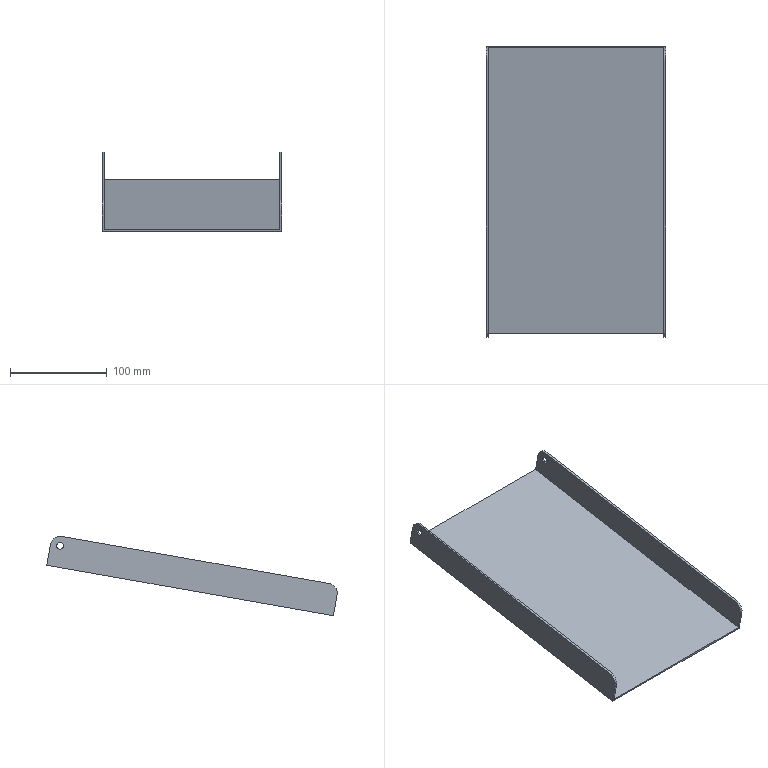Part | NX | features HB 2 | 1 solid | 16 faces | box 185 x 300.028 x 82.132 mm | volume 146980 mm3 | plane 10 | cylinder 6 | commonest cylinder face diameters 20 x4 7 x2
STEP:
#1=CARTESIAN_POINT('',(2913.,-963.709,-446.218));
#2=VERTEX_POINT('',#1);
#3=CARTESIAN_POINT('',(2913.,-687.349,-397.488));
#4=VERTEX_POINT('',#3);
#5=CARTESIAN_POINT('',(2913.,-562.892,-375.543));
#6=DIRECTION('',(0.,0.9848,0.1736));
#7=VECTOR('',#6,1000.);
#8=LINE('',#5,#7);
#9=EDGE_CURVE('',#2,#4,#8,.T.);
#10=ORIENTED_EDGE('',*,*,#9,.T.);
#11=CARTESIAN_POINT('',(2913.,-675.764,-405.6));
#12=VERTEX_POINT('',#11);
#13=CARTESIAN_POINT('',(2913.,-685.612,-407.336));
#14=DIRECTION('',(1.,0.,0.));
#15=DIRECTION('',(0.,-0.5736,0.8192));
#16=AXIS2_PLACEMENT_3D('',#13,#14,#15);
#17=CIRCLE('',#16,10.);
#18=EDGE_CURVE('',#12,#4,#17,.T.);
#19=ORIENTED_EDGE('',*,*,#18,.F.);
#20=CARTESIAN_POINT('',(2913.,-671.944,-427.266));
#21=VERTEX_POINT('',#20);
#22=CARTESIAN_POINT('',(2913.,-672.291,-425.296));
#23=DIRECTION('',(0.,-0.1736,0.9848));
#24=VECTOR('',#23,1000.);
#25=LINE('',#22,#24);
#26=EDGE_CURVE('',#21,#12,#25,.T.);
#27=ORIENTED_EDGE('',*,*,#26,.F.);
#28=CARTESIAN_POINT('',(2913.,-968.,-479.468));
#29=VERTEX_POINT('',#28);
#30=CARTESIAN_POINT('',(2913.,-557.335,-407.057));
#31=DIRECTION('',(0.,-0.9848,-0.1736));
#32=VECTOR('',#31,1000.);
#33=LINE('',#30,#32);
#34=EDGE_CURVE('',#21,#29,#33,.T.);
#35=ORIENTED_EDGE('',*,*,#34,.T.);
#36=CARTESIAN_POINT('',(2913.,-971.82,-457.803));
#37=VERTEX_POINT('',#36);
#38=CARTESIAN_POINT('',(2913.,-968.347,-477.499));
#39=DIRECTION('',(0.,-0.1736,0.9848));
#40=VECTOR('',#39,1000.);
#41=LINE('',#38,#40);
#42=EDGE_CURVE('',#29,#37,#41,.T.);
#43=ORIENTED_EDGE('',*,*,#42,.T.);
#44=CARTESIAN_POINT('',(2913.,-961.972,-456.066));
#45=DIRECTION('',(-1.,0.,0.));
#46=DIRECTION('',(0.,0.2588,0.9659));
#47=AXIS2_PLACEMENT_3D('',#44,#45,#46);
#48=CIRCLE('',#47,10.);
#49=EDGE_CURVE('',#37,#2,#48,.T.);
#50=ORIENTED_EDGE('',*,*,#49,.T.);
#51=EDGE_LOOP('',(#10,#19,#27,#35,#43,#50));
#52=FACE_BOUND('',#51,.T.);
#53=CARTESIAN_POINT('',(2913.,-684.707,-403.956));
#54=VERTEX_POINT('',#53);
#55=CARTESIAN_POINT('',(2913.,-685.612,-407.336));
#56=DIRECTION('',(1.,0.,0.));
#57=DIRECTION('',(0.,0.2588,0.9659));
#58=AXIS2_PLACEMENT_3D('',#55,#56,#57);
#59=CIRCLE('',#58,3.5);
#60=EDGE_CURVE('',#54,#54,#59,.T.);
#61=ORIENTED_EDGE('',*,*,#60,.T.);
#62=EDGE_LOOP('',(#61));
#63=FACE_BOUND('',#62,.T.);
#64=CARTESIAN_POINT('',(2913.,-557.683,-405.087));
#65=DIRECTION('',(1.,0.,0.));
#66=DIRECTION('',(0.,-0.2588,-0.9659));
#67=AXIS2_PLACEMENT_3D('',#64,#65,#66);
#68=PLANE('',#67);
#69=ADVANCED_FACE('',(#52,#63),#68,.F.);
#70=CARTESIAN_POINT('',(2915.,-963.709,-446.218));
#71=VERTEX_POINT('',#70);
#72=CARTESIAN_POINT('',(2915.,-971.82,-457.803));
#73=VERTEX_POINT('',#72);
#74=CARTESIAN_POINT('',(2915.,-961.972,-456.066));
#75=DIRECTION('',(1.,0.,0.));
#76=DIRECTION('',(0.,0.2588,0.9659));
#77=AXIS2_PLACEMENT_3D('',#74,#75,#76);
#78=CIRCLE('',#77,10.);
#79=EDGE_CURVE('',#71,#73,#78,.T.);
#80=ORIENTED_EDGE('',*,*,#79,.T.);
#81=CARTESIAN_POINT('',(2915.,-968.347,-477.499));
#82=VERTEX_POINT('',#81);
#83=CARTESIAN_POINT('',(2915.,-968.347,-477.499));
#84=DIRECTION('',(0.,-0.1736,0.9848));
#85=VECTOR('',#84,1000.);
#86=LINE('',#83,#85);
#87=EDGE_CURVE('',#82,#73,#86,.T.);
#88=ORIENTED_EDGE('',*,*,#87,.F.);
#89=CARTESIAN_POINT('',(2915.,-672.291,-425.296));
#90=VERTEX_POINT('',#89);
#91=CARTESIAN_POINT('',(2915.,-557.683,-405.087));
#92=DIRECTION('',(0.,0.9848,0.1736));
#93=VECTOR('',#92,1000.);
#94=LINE('',#91,#93);
#95=EDGE_CURVE('',#82,#90,#94,.T.);
#96=ORIENTED_EDGE('',*,*,#95,.T.);
#97=CARTESIAN_POINT('',(2915.,-675.764,-405.6));
#98=VERTEX_POINT('',#97);
#99=CARTESIAN_POINT('',(2915.,-672.291,-425.296));
#100=DIRECTION('',(0.,-0.1736,0.9848));
#101=VECTOR('',#100,1000.);
#102=LINE('',#99,#101);
#103=EDGE_CURVE('',#90,#98,#102,.T.);
#104=ORIENTED_EDGE('',*,*,#103,.T.);
#105=CARTESIAN_POINT('',(2915.,-687.349,-397.488));
#106=VERTEX_POINT('',#105);
#107=CARTESIAN_POINT('',(2915.,-685.612,-407.336));
#108=DIRECTION('',(-1.,0.,0.));
#109=DIRECTION('',(0.,-0.5736,0.8192));
#110=AXIS2_PLACEMENT_3D('',#107,#108,#109);
#111=CIRCLE('',#110,10.);
#112=EDGE_CURVE('',#106,#98,#111,.T.);
#113=ORIENTED_EDGE('',*,*,#112,.F.);
#114=CARTESIAN_POINT('',(2915.,-562.892,-375.543));
#115=DIRECTION('',(0.,0.9848,0.1736));
#116=VECTOR('',#115,1000.);
#117=LINE('',#114,#116);
#118=EDGE_CURVE('',#71,#106,#117,.T.);
#119=ORIENTED_EDGE('',*,*,#118,.F.);
#120=EDGE_LOOP('',(#80,#88,#96,#104,#113,#119));
#121=FACE_BOUND('',#120,.T.);
#122=CARTESIAN_POINT('',(2915.,-684.707,-403.956));
#123=VERTEX_POINT('',#122);
#124=CARTESIAN_POINT('',(2915.,-685.612,-407.336));
#125=DIRECTION('',(-1.,0.,0.));
#126=DIRECTION('',(0.,0.2588,0.9659));
#127=AXIS2_PLACEMENT_3D('',#124,#125,#126);
#128=CIRCLE('',#127,3.5);
#129=EDGE_CURVE('',#123,#123,#128,.T.);
#130=ORIENTED_EDGE('',*,*,#129,.T.);
#131=EDGE_LOOP('',(#130));
#132=FACE_BOUND('',#131,.T.);
#133=CARTESIAN_POINT('',(2915.,-557.683,-405.087));
#134=DIRECTION('',(1.,0.,0.));
#135=DIRECTION('',(0.,0.2588,0.9659));
#136=AXIS2_PLACEMENT_3D('',#133,#134,#135);
#137=PLANE('',#136);
#138=ADVANCED_FACE('',(#121,#132),#137,.T.);
#139=CARTESIAN_POINT('',(3098.,-686.518,-410.717));
#140=VERTEX_POINT('',#139);
#141=CARTESIAN_POINT('',(3098.,-685.612,-407.336));
#142=DIRECTION('',(-1.,0.,0.));
#143=DIRECTION('',(0.,-0.2588,-0.9659));
#144=AXIS2_PLACEMENT_3D('',#141,#142,#143);
#145=CIRCLE('',#144,3.5);
#146=EDGE_CURVE('',#140,#140,#145,.T.);
#147=ORIENTED_EDGE('',*,*,#146,.T.);
#148=EDGE_LOOP('',(#147));
#149=FACE_BOUND('',#148,.T.);
#150=CARTESIAN_POINT('',(3098.,-968.,-479.468));
#151=VERTEX_POINT('',#150);
#152=CARTESIAN_POINT('',(3098.,-671.944,-427.266));
#153=VERTEX_POINT('',#152);
#154=CARTESIAN_POINT('',(3098.,-557.335,-407.057));
#155=DIRECTION('',(0.,0.9848,0.1736));
#156=VECTOR('',#155,1000.);
#157=LINE('',#154,#156);
#158=EDGE_CURVE('',#151,#153,#157,.T.);
#159=ORIENTED_EDGE('',*,*,#158,.T.);
#160=CARTESIAN_POINT('',(3098.,-675.764,-405.6));
#161=VERTEX_POINT('',#160);
#162=CARTESIAN_POINT('',(3098.,-672.291,-425.296));
#163=DIRECTION('',(0.,-0.1736,0.9848));
#164=VECTOR('',#163,1000.);
#165=LINE('',#162,#164);
#166=EDGE_CURVE('',#153,#161,#165,.T.);
#167=ORIENTED_EDGE('',*,*,#166,.T.);
#168=CARTESIAN_POINT('',(3098.,-687.349,-397.488));
#169=VERTEX_POINT('',#168);
#170=CARTESIAN_POINT('',(3098.,-685.612,-407.336));
#171=DIRECTION('',(-1.,0.,0.));
#172=DIRECTION('',(0.,0.5736,-0.8192));
#173=AXIS2_PLACEMENT_3D('',#170,#171,#172);
#174=CIRCLE('',#173,10.);
#175=EDGE_CURVE('',#169,#161,#174,.T.);
#176=ORIENTED_EDGE('',*,*,#175,.F.);
#177=CARTESIAN_POINT('',(3098.,-963.709,-446.218));
#178=VERTEX_POINT('',#177);
#179=CARTESIAN_POINT('',(3098.,-562.892,-375.543));
#180=DIRECTION('',(0.,0.9848,0.1736));
#181=VECTOR('',#180,1000.);
#182=LINE('',#179,#181);
#183=EDGE_CURVE('',#178,#169,#182,.T.);
#184=ORIENTED_EDGE('',*,*,#183,.F.);
#185=CARTESIAN_POINT('',(3098.,-971.82,-457.803));
#186=VERTEX_POINT('',#185);
#187=CARTESIAN_POINT('',(3098.,-961.972,-456.066));
#188=DIRECTION('',(1.,0.,0.));
#189=DIRECTION('',(0.,-0.2588,-0.9659));
#190=AXIS2_PLACEMENT_3D('',#187,#188,#189);
#191=CIRCLE('',#190,10.);
#192=EDGE_CURVE('',#178,#186,#191,.T.);
#193=ORIENTED_EDGE('',*,*,#192,.T.);
#194=CARTESIAN_POINT('',(3098.,-968.347,-477.499));
#195=DIRECTION('',(0.,-0.1736,0.9848));
#196=VECTOR('',#195,1000.);
#197=LINE('',#194,#196);
#198=EDGE_CURVE('',#151,#186,#197,.T.);
#199=ORIENTED_EDGE('',*,*,#198,.F.);
#200=EDGE_LOOP('',(#159,#167,#176,#184,#193,#199));
#201=FACE_BOUND('',#200,.T.);
#202=CARTESIAN_POINT('',(3098.,-557.683,-405.087));
#203=DIRECTION('',(-1.,0.,0.));
#204=DIRECTION('',(0.,0.2588,0.9659));
#205=AXIS2_PLACEMENT_3D('',#202,#203,#204);
#206=PLANE('',#205);
#207=ADVANCED_FACE('',(#149,#201),#206,.F.);
#208=CARTESIAN_POINT('',(3096.,-968.347,-477.499));
#209=VERTEX_POINT('',#208);
#210=CARTESIAN_POINT('',(2994.,-968.347,-477.499));
#211=DIRECTION('',(1.,0.,0.));
#212=VECTOR('',#211,1000.);
#213=LINE('',#210,#212);
#214=EDGE_CURVE('',#82,#209,#213,.T.);
#215=ORIENTED_EDGE('',*,*,#214,.T.);
#216=CARTESIAN_POINT('',(3096.,-672.291,-425.296));
#217=VERTEX_POINT('',#216);
#218=CARTESIAN_POINT('',(3096.,-557.683,-405.087));
#219=DIRECTION('',(0.,-0.9848,-0.1736));
#220=VECTOR('',#219,1000.);
#221=LINE('',#218,#220);
#222=EDGE_CURVE('',#217,#209,#221,.T.);
#223=ORIENTED_EDGE('',*,*,#222,.F.);
#224=CARTESIAN_POINT('',(2994.,-672.291,-425.296));
#225=DIRECTION('',(1.,0.,0.));
#226=VECTOR('',#225,1000.);
#227=LINE('',#224,#226);
#228=EDGE_CURVE('',#90,#217,#227,.T.);
#229=ORIENTED_EDGE('',*,*,#228,.F.);
#230=ORIENTED_EDGE('',*,*,#95,.F.);
#231=EDGE_LOOP('',(#215,#223,#229,#230));
#232=FACE_BOUND('',#231,.T.);
#233=CARTESIAN_POINT('',(2994.,-557.683,-405.087));
#234=DIRECTION('',(0.,-0.1736,0.9848));
#235=DIRECTION('',(1.,0.,0.));
#236=AXIS2_PLACEMENT_3D('',#233,#234,#235);
#237=PLANE('',#236);
#238=ADVANCED_FACE('',(#232),#237,.T.);
#239=CARTESIAN_POINT('',(2994.,-671.944,-427.266));
#240=DIRECTION('',(1.,0.,0.));
#241=VECTOR('',#240,1000.);
#242=LINE('',#239,#241);
#243=EDGE_CURVE('',#21,#153,#242,.T.);
#244=ORIENTED_EDGE('',*,*,#243,.T.);
#245=ORIENTED_EDGE('',*,*,#158,.F.);
#246=CARTESIAN_POINT('',(2994.,-968.,-479.468));
#247=DIRECTION('',(1.,0.,0.));
#248=VECTOR('',#247,1000.);
#249=LINE('',#246,#248);
#250=EDGE_CURVE('',#29,#151,#249,.T.);
#251=ORIENTED_EDGE('',*,*,#250,.F.);
#252=ORIENTED_EDGE('',*,*,#34,.F.);
#253=EDGE_LOOP('',(#244,#245,#251,#252));
#254=FACE_BOUND('',#253,.T.);
#255=CARTESIAN_POINT('',(2994.,-557.335,-407.057));
#256=DIRECTION('',(0.,-0.1736,0.9848));
#257=DIRECTION('',(1.,0.,0.));
#258=AXIS2_PLACEMENT_3D('',#255,#256,#257);
#259=PLANE('',#258);
#260=ADVANCED_FACE('',(#254),#259,.F.);
#261=ORIENTED_EDGE('',*,*,#183,.T.);
#262=CARTESIAN_POINT('',(3096.,-687.349,-397.488));
#263=VERTEX_POINT('',#262);
#264=CARTESIAN_POINT('',(3226.,-687.349,-397.488));
#265=DIRECTION('',(1.,0.,0.));
#266=VECTOR('',#265,1000.);
#267=LINE('',#264,#266);
#268=EDGE_CURVE('',#263,#169,#267,.T.);
#269=ORIENTED_EDGE('',*,*,#268,.F.);
#270=CARTESIAN_POINT('',(3096.,-963.709,-446.218));
#271=VERTEX_POINT('',#270);
#272=CARTESIAN_POINT('',(3096.,-562.892,-375.543));
#273=DIRECTION('',(0.,0.9848,0.1736));
#274=VECTOR('',#273,1000.);
#275=LINE('',#272,#274);
#276=EDGE_CURVE('',#271,#263,#275,.T.);
#277=ORIENTED_EDGE('',*,*,#276,.F.);
#278=CARTESIAN_POINT('',(3226.,-963.709,-446.218));
#279=DIRECTION('',(1.,0.,0.));
#280=VECTOR('',#279,1000.);
#281=LINE('',#278,#280);
#282=EDGE_CURVE('',#271,#178,#281,.T.);
#283=ORIENTED_EDGE('',*,*,#282,.T.);
#284=EDGE_LOOP('',(#261,#269,#277,#283));
#285=FACE_BOUND('',#284,.T.);
#286=CARTESIAN_POINT('',(3226.,-562.892,-375.543));
#287=DIRECTION('',(0.,0.1736,-0.9848));
#288=DIRECTION('',(0.,-0.9848,-0.1736));
#289=AXIS2_PLACEMENT_3D('',#286,#287,#288);
#290=PLANE('',#289);
#291=ADVANCED_FACE('',(#285),#290,.F.);
#292=CARTESIAN_POINT('',(3096.,-686.518,-410.717));
#293=VERTEX_POINT('',#292);
#294=CARTESIAN_POINT('',(3096.,-685.612,-407.336));
#295=DIRECTION('',(-1.,0.,0.));
#296=DIRECTION('',(0.,-0.2588,-0.9659));
#297=AXIS2_PLACEMENT_3D('',#294,#295,#296);
#298=CIRCLE('',#297,3.5);
#299=EDGE_CURVE('',#293,#293,#298,.T.);
#300=ORIENTED_EDGE('',*,*,#299,.F.);
#301=EDGE_LOOP('',(#300));
#302=FACE_BOUND('',#301,.T.);
#303=ORIENTED_EDGE('',*,*,#222,.T.);
#304=CARTESIAN_POINT('',(3096.,-971.82,-457.803));
#305=VERTEX_POINT('',#304);
#306=CARTESIAN_POINT('',(3096.,-968.347,-477.499));
#307=DIRECTION('',(0.,-0.1736,0.9848));
#308=VECTOR('',#307,1000.);
#309=LINE('',#306,#308);
#310=EDGE_CURVE('',#209,#305,#309,.T.);
#311=ORIENTED_EDGE('',*,*,#310,.T.);
#312=CARTESIAN_POINT('',(3096.,-961.972,-456.066));
#313=DIRECTION('',(-1.,0.,0.));
#314=DIRECTION('',(0.,-0.2588,-0.9659));
#315=AXIS2_PLACEMENT_3D('',#312,#313,#314);
#316=CIRCLE('',#315,10.);
#317=EDGE_CURVE('',#305,#271,#316,.T.);
#318=ORIENTED_EDGE('',*,*,#317,.T.);
#319=ORIENTED_EDGE('',*,*,#276,.T.);
#320=CARTESIAN_POINT('',(3096.,-675.764,-405.6));
#321=VERTEX_POINT('',#320);
#322=CARTESIAN_POINT('',(3096.,-685.612,-407.336));
#323=DIRECTION('',(1.,0.,0.));
#324=DIRECTION('',(0.,0.5736,-0.8192));
#325=AXIS2_PLACEMENT_3D('',#322,#323,#324);
#326=CIRCLE('',#325,10.);
#327=EDGE_CURVE('',#321,#263,#326,.T.);
#328=ORIENTED_EDGE('',*,*,#327,.F.);
#329=CARTESIAN_POINT('',(3096.,-672.291,-425.296));
#330=DIRECTION('',(0.,-0.1736,0.9848));
#331=VECTOR('',#330,1000.);
#332=LINE('',#329,#331);
#333=EDGE_CURVE('',#217,#321,#332,.T.);
#334=ORIENTED_EDGE('',*,*,#333,.F.);
#335=EDGE_LOOP('',(#303,#311,#318,#319,#328,#334));
#336=FACE_BOUND('',#335,.T.);
#337=CARTESIAN_POINT('',(3096.,-557.683,-405.087));
#338=DIRECTION('',(-1.,0.,0.));
#339=DIRECTION('',(0.,0.2588,0.9659));
#340=AXIS2_PLACEMENT_3D('',#337,#338,#339);
#341=PLANE('',#340);
#342=ADVANCED_FACE('',(#302,#336),#341,.T.);
#343=ORIENTED_EDGE('',*,*,#118,.T.);
#344=CARTESIAN_POINT('',(2929.,-687.349,-397.488));
#345=DIRECTION('',(1.,0.,0.));
#346=VECTOR('',#345,1000.);
#347=LINE('',#344,#346);
#348=EDGE_CURVE('',#4,#106,#347,.T.);
#349=ORIENTED_EDGE('',*,*,#348,.F.);
#350=ORIENTED_EDGE('',*,*,#9,.F.);
#351=CARTESIAN_POINT('',(2929.,-963.709,-446.218));
#352=DIRECTION('',(1.,0.,0.));
#353=VECTOR('',#352,1000.);
#354=LINE('',#351,#353);
#355=EDGE_CURVE('',#2,#71,#354,.T.);
#356=ORIENTED_EDGE('',*,*,#355,.T.);
#357=EDGE_LOOP('',(#343,#349,#350,#356));
#358=FACE_BOUND('',#357,.T.);
#359=CARTESIAN_POINT('',(2929.,-562.892,-375.543));
#360=DIRECTION('',(0.,0.1736,-0.9848));
#361=DIRECTION('',(0.,-0.9848,-0.1736));
#362=AXIS2_PLACEMENT_3D('',#359,#360,#361);
#363=PLANE('',#362);
#364=ADVANCED_FACE('',(#358),#363,.F.);
#365=ORIENTED_EDGE('',*,*,#42,.F.);
#366=ORIENTED_EDGE('',*,*,#250,.T.);
#367=ORIENTED_EDGE('',*,*,#198,.T.);
#368=CARTESIAN_POINT('',(2994.,-971.82,-457.803));
#369=DIRECTION('',(-1.,0.,0.));
#370=VECTOR('',#369,1000.);
#371=LINE('',#368,#370);
#372=EDGE_CURVE('',#186,#305,#371,.T.);
#373=ORIENTED_EDGE('',*,*,#372,.T.);
#374=ORIENTED_EDGE('',*,*,#310,.F.);
#375=ORIENTED_EDGE('',*,*,#214,.F.);
#376=ORIENTED_EDGE('',*,*,#87,.T.);
#377=CARTESIAN_POINT('',(2994.,-971.82,-457.803));
#378=DIRECTION('',(-1.,0.,0.));
#379=VECTOR('',#378,1000.);
#380=LINE('',#377,#379);
#381=EDGE_CURVE('',#73,#37,#380,.T.);
#382=ORIENTED_EDGE('',*,*,#381,.T.);
#383=EDGE_LOOP('',(#365,#366,#367,#373,#374,#375,#376,#382));
#384=FACE_BOUND('',#383,.T.);
#385=CARTESIAN_POINT('',(2994.,-968.347,-477.499));
#386=DIRECTION('',(0.,0.9848,0.1736));
#387=DIRECTION('',(0.,0.1736,-0.9848));
#388=AXIS2_PLACEMENT_3D('',#385,#386,#387);
#389=PLANE('',#388);
#390=ADVANCED_FACE('',(#384),#389,.F.);
#391=ORIENTED_EDGE('',*,*,#79,.F.);
#392=ORIENTED_EDGE('',*,*,#355,.F.);
#393=ORIENTED_EDGE('',*,*,#49,.F.);
#394=ORIENTED_EDGE('',*,*,#381,.F.);
#395=EDGE_LOOP('',(#391,#392,#393,#394));
#396=FACE_BOUND('',#395,.T.);
#397=CARTESIAN_POINT('',(2929.,-961.972,-456.066));
#398=DIRECTION('',(-1.,0.,0.));
#399=DIRECTION('',(0.,0.2588,0.9659));
#400=AXIS2_PLACEMENT_3D('',#397,#398,#399);
#401=CYLINDRICAL_SURFACE('',#400,10.);
#402=ADVANCED_FACE('',(#396),#401,.T.);
#403=ORIENTED_EDGE('',*,*,#317,.F.);
#404=ORIENTED_EDGE('',*,*,#372,.F.);
#405=ORIENTED_EDGE('',*,*,#192,.F.);
#406=ORIENTED_EDGE('',*,*,#282,.F.);
#407=EDGE_LOOP('',(#403,#404,#405,#406));
#408=FACE_BOUND('',#407,.T.);
#409=CARTESIAN_POINT('',(2968.,-961.972,-456.066));
#410=DIRECTION('',(1.,0.,0.));
#411=DIRECTION('',(0.,-0.2588,-0.9659));
#412=AXIS2_PLACEMENT_3D('',#409,#410,#411);
#413=CYLINDRICAL_SURFACE('',#412,10.);
#414=ADVANCED_FACE('',(#408),#413,.T.);
#415=ORIENTED_EDGE('',*,*,#26,.T.);
#416=CARTESIAN_POINT('',(2929.,-675.764,-405.6));
#417=DIRECTION('',(-1.,0.,0.));
#418=VECTOR('',#417,1000.);
#419=LINE('',#416,#418);
#420=EDGE_CURVE('',#98,#12,#419,.T.);
#421=ORIENTED_EDGE('',*,*,#420,.F.);
#422=ORIENTED_EDGE('',*,*,#103,.F.);
#423=ORIENTED_EDGE('',*,*,#228,.T.);
#424=ORIENTED_EDGE('',*,*,#333,.T.);
#425=CARTESIAN_POINT('',(2968.,-675.764,-405.6));
#426=DIRECTION('',(-1.,0.,0.));
#427=VECTOR('',#426,1000.);
#428=LINE('',#425,#427);
#429=EDGE_CURVE('',#161,#321,#428,.T.);
#430=ORIENTED_EDGE('',*,*,#429,.F.);
#431=ORIENTED_EDGE('',*,*,#166,.F.);
#432=ORIENTED_EDGE('',*,*,#243,.F.);
#433=EDGE_LOOP('',(#415,#421,#422,#423,#424,#430,#431,#432));
#434=FACE_BOUND('',#433,.T.);
#435=CARTESIAN_POINT('',(2994.,-672.291,-425.296));
#436=DIRECTION('',(0.,-0.9848,-0.1736));
#437=DIRECTION('',(0.,0.1736,-0.9848));
#438=AXIS2_PLACEMENT_3D('',#435,#436,#437);
#439=PLANE('',#438);
#440=ADVANCED_FACE('',(#434),#439,.F.);
#441=ORIENTED_EDGE('',*,*,#112,.T.);
#442=ORIENTED_EDGE('',*,*,#420,.T.);
#443=ORIENTED_EDGE('',*,*,#18,.T.);
#444=ORIENTED_EDGE('',*,*,#348,.T.);
#445=EDGE_LOOP('',(#441,#442,#443,#444));
#446=FACE_BOUND('',#445,.T.);
#447=CARTESIAN_POINT('',(2929.,-685.612,-407.336));
#448=DIRECTION('',(-1.,0.,0.));
#449=DIRECTION('',(0.,-0.5736,0.8192));
#450=AXIS2_PLACEMENT_3D('',#447,#448,#449);
#451=CYLINDRICAL_SURFACE('',#450,10.);
#452=ADVANCED_FACE('',(#446),#451,.T.);
#453=ORIENTED_EDGE('',*,*,#327,.T.);
#454=ORIENTED_EDGE('',*,*,#268,.T.);
#455=ORIENTED_EDGE('',*,*,#175,.T.);
#456=ORIENTED_EDGE('',*,*,#429,.T.);
#457=EDGE_LOOP('',(#453,#454,#455,#456));
#458=FACE_BOUND('',#457,.T.);
#459=CARTESIAN_POINT('',(2968.,-685.612,-407.336));
#460=DIRECTION('',(1.,0.,0.));
#461=DIRECTION('',(0.,0.5736,-0.8192));
#462=AXIS2_PLACEMENT_3D('',#459,#460,#461);
#463=CYLINDRICAL_SURFACE('',#462,10.);
#464=ADVANCED_FACE('',(#458),#463,.T.);
#465=ORIENTED_EDGE('',*,*,#299,.T.);
#466=EDGE_LOOP('',(#465));
#467=FACE_BOUND('',#466,.T.);
#468=ORIENTED_EDGE('',*,*,#146,.F.);
#469=EDGE_LOOP('',(#468));
#470=FACE_BOUND('',#469,.T.);
#471=CARTESIAN_POINT('',(3228.,-685.612,-407.336));
#472=DIRECTION('',(-1.,0.,0.));
#473=DIRECTION('',(0.,0.2588,0.9659));
#474=AXIS2_PLACEMENT_3D('',#471,#472,#473);
#475=CYLINDRICAL_SURFACE('',#474,3.5);
#476=ADVANCED_FACE('',(#467,#470),#475,.F.);
#477=ORIENTED_EDGE('',*,*,#129,.F.);
#478=EDGE_LOOP('',(#477));
#479=FACE_BOUND('',#478,.T.);
#480=ORIENTED_EDGE('',*,*,#60,.F.);
#481=EDGE_LOOP('',(#480));
#482=FACE_BOUND('',#481,.T.);
#483=CARTESIAN_POINT('',(2323.,-685.612,-407.336));
#484=DIRECTION('',(1.,0.,0.));
#485=DIRECTION('',(0.,-0.2588,-0.9659));
#486=AXIS2_PLACEMENT_3D('',#483,#484,#485);
#487=CYLINDRICAL_SURFACE('',#486,3.5);
#488=ADVANCED_FACE('',(#479,#482),#487,.F.);
#489=CLOSED_SHELL('',(#69,#138,#207,#238,#260,#291,#342,#364,#390,#402,#414,#440,#452,#464,#476,#488));
#490=MANIFOLD_SOLID_BREP('',#489);
#491=(LENGTH_UNIT()NAMED_UNIT(*)SI_UNIT(.MILLI.,.METRE.));
#492=UNCERTAINTY_MEASURE_WITH_UNIT(LENGTH_MEASURE(0.00001),#491,'','');
#493=(NAMED_UNIT(*)PLANE_ANGLE_UNIT()SI_UNIT($,.RADIAN.));
#494=(NAMED_UNIT(*)SI_UNIT($,.STERADIAN.)SOLID_ANGLE_UNIT());
#495=(GEOMETRIC_REPRESENTATION_CONTEXT(3)GLOBAL_UNCERTAINTY_ASSIGNED_CONTEXT((#492))GLOBAL_UNIT_ASSIGNED_CONTEXT((#491,#493,#494))REPRESENTATION_CONTEXT('',''));
#496=ADVANCED_BREP_SHAPE_REPRESENTATION('',(#490),#495);